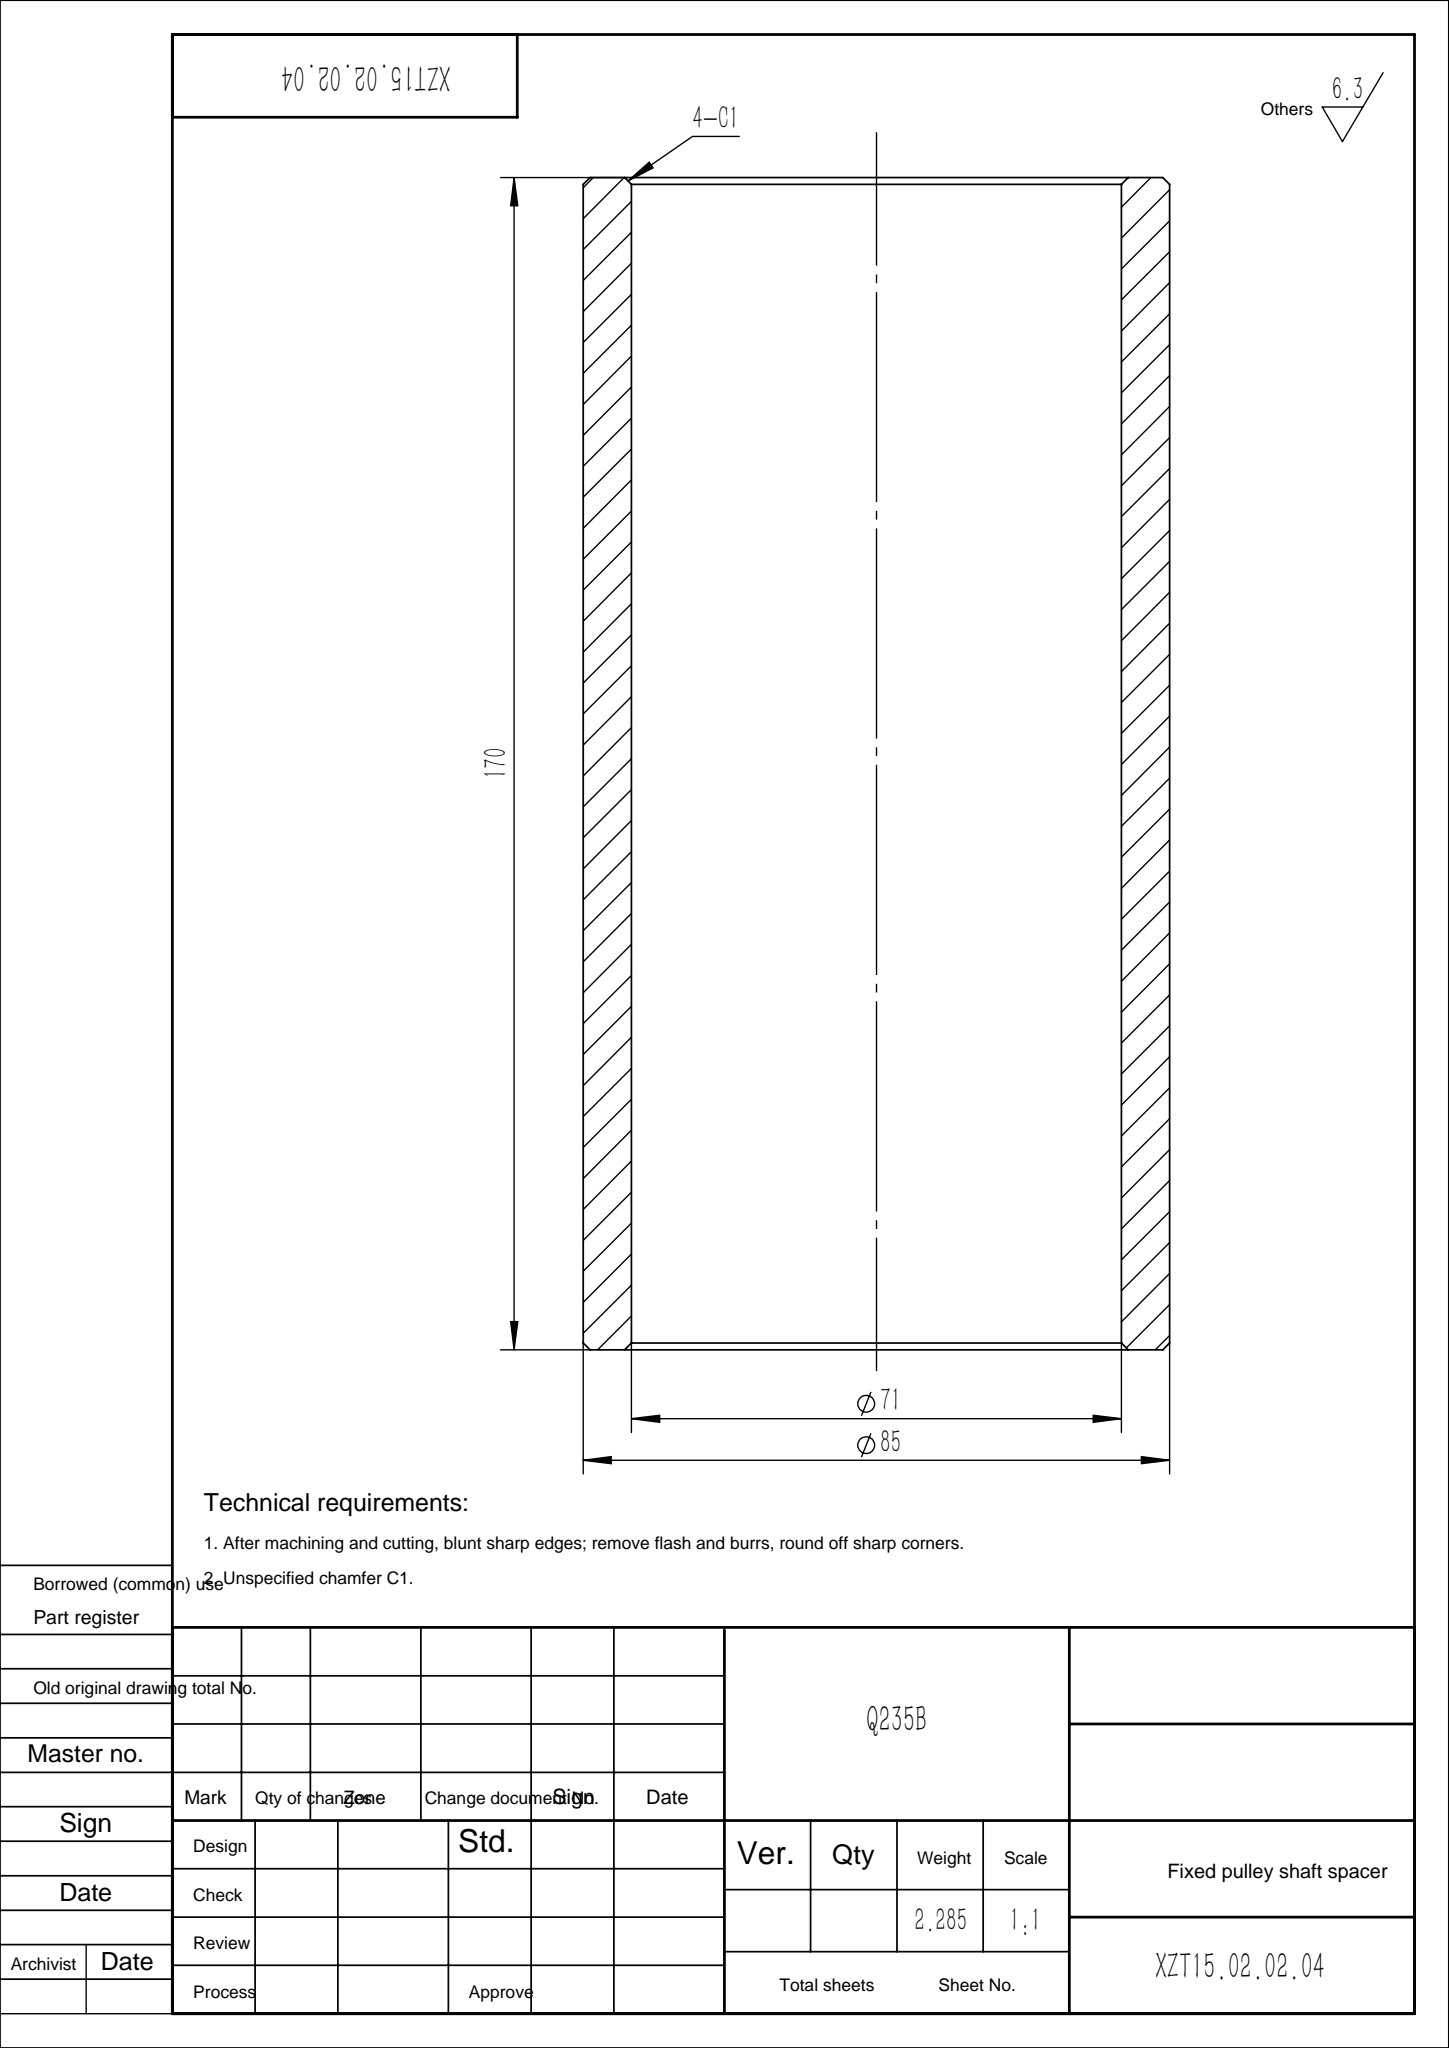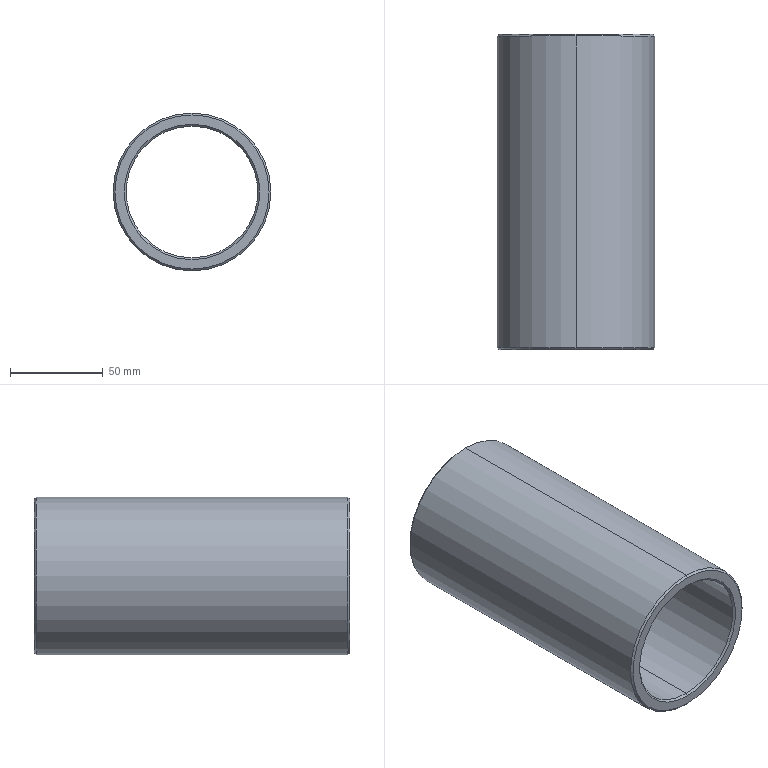Part | SolidWorks | features Chamfer 1, Extrusion 1 | 1 solid | 14 faces | box 85 x 170 x 85 mm | volume 291113 mm3 | cone 8 | cylinder 4 | plane 2 | commonest cylinder face diameters 71 x2 85 x2
STEP:
#1=CARTESIAN_POINT('',(0.,170.,41.5));
#2=VERTEX_POINT('',#1);
#3=CARTESIAN_POINT('',(0.,170.,-41.5));
#4=VERTEX_POINT('',#3);
#5=CARTESIAN_POINT('',(0.,170.,0.));
#6=DIRECTION('',(0.,1.,0.));
#7=DIRECTION('',(0.,0.,1.));
#8=AXIS2_PLACEMENT_3D('',#5,#6,#7);
#9=CIRCLE('',#8,41.5);
#10=EDGE_CURVE('',#2,#4,#9,.T.);
#11=ORIENTED_EDGE('',*,*,#10,.F.);
#12=CARTESIAN_POINT('',(0.,169.,42.5));
#13=VERTEX_POINT('',#12);
#14=CARTESIAN_POINT('',(0.,170.,41.5));
#15=DIRECTION('',(0.,-0.7071,0.7071));
#16=VECTOR('',#15,1000.);
#17=LINE('',#14,#16);
#18=EDGE_CURVE('',#2,#13,#17,.T.);
#19=ORIENTED_EDGE('',*,*,#18,.T.);
#20=CARTESIAN_POINT('',(0.,169.,-42.5));
#21=VERTEX_POINT('',#20);
#22=CARTESIAN_POINT('',(0.,169.,0.));
#23=DIRECTION('',(0.,-1.,0.));
#24=DIRECTION('',(0.,0.,1.));
#25=AXIS2_PLACEMENT_3D('',#22,#23,#24);
#26=CIRCLE('',#25,42.5);
#27=EDGE_CURVE('',#21,#13,#26,.T.);
#28=ORIENTED_EDGE('',*,*,#27,.F.);
#29=CARTESIAN_POINT('',(0.,170.,-41.5));
#30=DIRECTION('',(0.,-0.7071,-0.7071));
#31=VECTOR('',#30,1000.);
#32=LINE('',#29,#31);
#33=EDGE_CURVE('',#4,#21,#32,.T.);
#34=ORIENTED_EDGE('',*,*,#33,.F.);
#35=EDGE_LOOP('',(#11,#19,#28,#34));
#36=FACE_OUTER_BOUND('',#35,.T.);
#37=CARTESIAN_POINT('',(0.,170.,0.));
#38=DIRECTION('',(0.,-1.,0.));
#39=DIRECTION('',(0.,0.,-1.));
#40=AXIS2_PLACEMENT_3D('',#37,#38,#39);
#41=CONICAL_SURFACE('',#40,41.5,0.7854);
#42=ADVANCED_FACE('',(#36),#41,.T.);
#43=CARTESIAN_POINT('',(0.,0.,-41.5));
#44=VERTEX_POINT('',#43);
#45=CARTESIAN_POINT('',(0.,0.,41.5));
#46=VERTEX_POINT('',#45);
#47=CARTESIAN_POINT('',(0.,0.,0.));
#48=DIRECTION('',(0.,-1.,0.));
#49=DIRECTION('',(0.,0.,1.));
#50=AXIS2_PLACEMENT_3D('',#47,#48,#49);
#51=CIRCLE('',#50,41.5);
#52=EDGE_CURVE('',#44,#46,#51,.T.);
#53=ORIENTED_EDGE('',*,*,#52,.F.);
#54=CARTESIAN_POINT('',(0.,1.,-42.5));
#55=VERTEX_POINT('',#54);
#56=CARTESIAN_POINT('',(0.,1.,-42.5));
#57=DIRECTION('',(0.,0.7071,-0.7071));
#58=VECTOR('',#57,1000.);
#59=LINE('',#56,#58);
#60=EDGE_CURVE('',#44,#55,#59,.T.);
#61=ORIENTED_EDGE('',*,*,#60,.T.);
#62=CARTESIAN_POINT('',(0.,1.,42.5));
#63=VERTEX_POINT('',#62);
#64=CARTESIAN_POINT('',(0.,1.,0.));
#65=DIRECTION('',(0.,1.,0.));
#66=DIRECTION('',(0.,0.,1.));
#67=AXIS2_PLACEMENT_3D('',#64,#65,#66);
#68=CIRCLE('',#67,42.5);
#69=EDGE_CURVE('',#63,#55,#68,.T.);
#70=ORIENTED_EDGE('',*,*,#69,.F.);
#71=CARTESIAN_POINT('',(0.,1.,42.5));
#72=DIRECTION('',(0.,0.7071,0.7071));
#73=VECTOR('',#72,1000.);
#74=LINE('',#71,#73);
#75=EDGE_CURVE('',#46,#63,#74,.T.);
#76=ORIENTED_EDGE('',*,*,#75,.F.);
#77=EDGE_LOOP('',(#53,#61,#70,#76));
#78=FACE_OUTER_BOUND('',#77,.T.);
#79=CARTESIAN_POINT('',(0.,1.,0.));
#80=DIRECTION('',(0.,1.,0.));
#81=DIRECTION('',(0.,0.,1.));
#82=AXIS2_PLACEMENT_3D('',#79,#80,#81);
#83=CONICAL_SURFACE('',#82,42.5,0.7854);
#84=ADVANCED_FACE('',(#78),#83,.T.);
#85=CARTESIAN_POINT('',(0.,169.,-35.5));
#86=VERTEX_POINT('',#85);
#87=CARTESIAN_POINT('',(0.,169.,35.5));
#88=VERTEX_POINT('',#87);
#89=CARTESIAN_POINT('',(0.,169.,0.));
#90=DIRECTION('',(0.,1.,0.));
#91=DIRECTION('',(0.,0.,1.));
#92=AXIS2_PLACEMENT_3D('',#89,#90,#91);
#93=CIRCLE('',#92,35.5);
#94=EDGE_CURVE('',#86,#88,#93,.T.);
#95=ORIENTED_EDGE('',*,*,#94,.F.);
#96=CARTESIAN_POINT('',(0.,170.,-36.5));
#97=VERTEX_POINT('',#96);
#98=CARTESIAN_POINT('',(0.,169.,-35.5));
#99=DIRECTION('',(0.,0.7071,-0.7071));
#100=VECTOR('',#99,1000.);
#101=LINE('',#98,#100);
#102=EDGE_CURVE('',#86,#97,#101,.T.);
#103=ORIENTED_EDGE('',*,*,#102,.T.);
#104=CARTESIAN_POINT('',(0.,170.,36.5));
#105=VERTEX_POINT('',#104);
#106=CARTESIAN_POINT('',(0.,170.,0.));
#107=DIRECTION('',(0.,-1.,0.));
#108=DIRECTION('',(0.,0.,1.));
#109=AXIS2_PLACEMENT_3D('',#106,#107,#108);
#110=CIRCLE('',#109,36.5);
#111=EDGE_CURVE('',#105,#97,#110,.T.);
#112=ORIENTED_EDGE('',*,*,#111,.F.);
#113=CARTESIAN_POINT('',(0.,169.,35.5));
#114=DIRECTION('',(0.,0.7071,0.7071));
#115=VECTOR('',#114,1000.);
#116=LINE('',#113,#115);
#117=EDGE_CURVE('',#88,#105,#116,.T.);
#118=ORIENTED_EDGE('',*,*,#117,.F.);
#119=EDGE_LOOP('',(#95,#103,#112,#118));
#120=FACE_OUTER_BOUND('',#119,.T.);
#121=CARTESIAN_POINT('',(0.,169.,0.));
#122=DIRECTION('',(0.,1.,0.));
#123=DIRECTION('',(0.,0.,1.));
#124=AXIS2_PLACEMENT_3D('',#121,#122,#123);
#125=CONICAL_SURFACE('',#124,35.5,0.7854);
#126=ADVANCED_FACE('',(#120),#125,.F.);
#127=CARTESIAN_POINT('',(0.,1.,35.5));
#128=VERTEX_POINT('',#127);
#129=CARTESIAN_POINT('',(0.,1.,-35.5));
#130=VERTEX_POINT('',#129);
#131=CARTESIAN_POINT('',(0.,1.,0.));
#132=DIRECTION('',(0.,-1.,0.));
#133=DIRECTION('',(0.,0.,1.));
#134=AXIS2_PLACEMENT_3D('',#131,#132,#133);
#135=CIRCLE('',#134,35.5);
#136=EDGE_CURVE('',#128,#130,#135,.T.);
#137=ORIENTED_EDGE('',*,*,#136,.F.);
#138=CARTESIAN_POINT('',(0.,0.,36.5));
#139=VERTEX_POINT('',#138);
#140=CARTESIAN_POINT('',(0.,0.,36.5));
#141=DIRECTION('',(0.,-0.7071,0.7071));
#142=VECTOR('',#141,1000.);
#143=LINE('',#140,#142);
#144=EDGE_CURVE('',#128,#139,#143,.T.);
#145=ORIENTED_EDGE('',*,*,#144,.T.);
#146=CARTESIAN_POINT('',(0.,0.,-36.5));
#147=VERTEX_POINT('',#146);
#148=CARTESIAN_POINT('',(0.,0.,0.));
#149=DIRECTION('',(0.,1.,0.));
#150=DIRECTION('',(0.,0.,1.));
#151=AXIS2_PLACEMENT_3D('',#148,#149,#150);
#152=CIRCLE('',#151,36.5);
#153=EDGE_CURVE('',#147,#139,#152,.T.);
#154=ORIENTED_EDGE('',*,*,#153,.F.);
#155=CARTESIAN_POINT('',(0.,0.,-36.5));
#156=DIRECTION('',(0.,-0.7071,-0.7071));
#157=VECTOR('',#156,1000.);
#158=LINE('',#155,#157);
#159=EDGE_CURVE('',#130,#147,#158,.T.);
#160=ORIENTED_EDGE('',*,*,#159,.F.);
#161=EDGE_LOOP('',(#137,#145,#154,#160));
#162=FACE_OUTER_BOUND('',#161,.T.);
#163=CARTESIAN_POINT('',(0.,0.,0.));
#164=DIRECTION('',(0.,-1.,0.));
#165=DIRECTION('',(0.,0.,-1.));
#166=AXIS2_PLACEMENT_3D('',#163,#164,#165);
#167=CONICAL_SURFACE('',#166,36.5,0.7854);
#168=ADVANCED_FACE('',(#162),#167,.F.);
#169=ORIENTED_EDGE('',*,*,#94,.T.);
#170=CARTESIAN_POINT('',(0.,170.,35.5));
#171=DIRECTION('',(0.,-1.,0.));
#172=VECTOR('',#171,1000.);
#173=LINE('',#170,#172);
#174=EDGE_CURVE('',#88,#128,#173,.T.);
#175=ORIENTED_EDGE('',*,*,#174,.T.);
#176=ORIENTED_EDGE('',*,*,#136,.T.);
#177=CARTESIAN_POINT('',(0.,170.,-35.5));
#178=DIRECTION('',(0.,-1.,0.));
#179=VECTOR('',#178,1000.);
#180=LINE('',#177,#179);
#181=EDGE_CURVE('',#86,#130,#180,.T.);
#182=ORIENTED_EDGE('',*,*,#181,.F.);
#183=EDGE_LOOP('',(#169,#175,#176,#182));
#184=FACE_OUTER_BOUND('',#183,.T.);
#185=CARTESIAN_POINT('',(0.,170.,0.));
#186=DIRECTION('',(0.,-1.,0.));
#187=DIRECTION('',(0.,0.,-1.));
#188=AXIS2_PLACEMENT_3D('',#185,#186,#187);
#189=CYLINDRICAL_SURFACE('',#188,35.5);
#190=ADVANCED_FACE('',(#184),#189,.F.);
#191=ORIENTED_EDGE('',*,*,#27,.T.);
#192=CARTESIAN_POINT('',(0.,170.,42.5));
#193=DIRECTION('',(0.,-1.,0.));
#194=VECTOR('',#193,1000.);
#195=LINE('',#192,#194);
#196=EDGE_CURVE('',#13,#63,#195,.T.);
#197=ORIENTED_EDGE('',*,*,#196,.T.);
#198=ORIENTED_EDGE('',*,*,#69,.T.);
#199=CARTESIAN_POINT('',(0.,170.,-42.5));
#200=DIRECTION('',(0.,-1.,0.));
#201=VECTOR('',#200,1000.);
#202=LINE('',#199,#201);
#203=EDGE_CURVE('',#21,#55,#202,.T.);
#204=ORIENTED_EDGE('',*,*,#203,.F.);
#205=EDGE_LOOP('',(#191,#197,#198,#204));
#206=FACE_OUTER_BOUND('',#205,.T.);
#207=CARTESIAN_POINT('',(0.,170.,0.));
#208=DIRECTION('',(0.,-1.,0.));
#209=DIRECTION('',(0.,0.,-1.));
#210=AXIS2_PLACEMENT_3D('',#207,#208,#209);
#211=CYLINDRICAL_SURFACE('',#210,42.5);
#212=ADVANCED_FACE('',(#206),#211,.T.);
#213=ORIENTED_EDGE('',*,*,#111,.T.);
#214=CARTESIAN_POINT('',(0.,170.,0.));
#215=DIRECTION('',(0.,-1.,0.));
#216=DIRECTION('',(0.,0.,1.));
#217=AXIS2_PLACEMENT_3D('',#214,#215,#216);
#218=CIRCLE('',#217,36.5);
#219=EDGE_CURVE('',#97,#105,#218,.T.);
#220=ORIENTED_EDGE('',*,*,#219,.T.);
#221=EDGE_LOOP('',(#213,#220));
#222=FACE_BOUND('',#221,.T.);
#223=CARTESIAN_POINT('',(0.,170.,0.));
#224=DIRECTION('',(0.,1.,0.));
#225=DIRECTION('',(0.,0.,1.));
#226=AXIS2_PLACEMENT_3D('',#223,#224,#225);
#227=CIRCLE('',#226,41.5);
#228=EDGE_CURVE('',#4,#2,#227,.T.);
#229=ORIENTED_EDGE('',*,*,#228,.T.);
#230=ORIENTED_EDGE('',*,*,#10,.T.);
#231=EDGE_LOOP('',(#229,#230));
#232=FACE_OUTER_BOUND('',#231,.T.);
#233=CARTESIAN_POINT('',(0.,170.,0.));
#234=DIRECTION('',(0.,1.,0.));
#235=DIRECTION('',(0.,0.,1.));
#236=AXIS2_PLACEMENT_3D('',#233,#234,#235);
#237=PLANE('',#236);
#238=ADVANCED_FACE('',(#222,#232),#237,.T.);
#239=ORIENTED_EDGE('',*,*,#153,.T.);
#240=CARTESIAN_POINT('',(0.,0.,0.));
#241=DIRECTION('',(0.,1.,0.));
#242=DIRECTION('',(0.,0.,1.));
#243=AXIS2_PLACEMENT_3D('',#240,#241,#242);
#244=CIRCLE('',#243,36.5);
#245=EDGE_CURVE('',#139,#147,#244,.T.);
#246=ORIENTED_EDGE('',*,*,#245,.T.);
#247=EDGE_LOOP('',(#239,#246));
#248=FACE_BOUND('',#247,.T.);
#249=CARTESIAN_POINT('',(0.,0.,0.));
#250=DIRECTION('',(0.,-1.,0.));
#251=DIRECTION('',(0.,0.,1.));
#252=AXIS2_PLACEMENT_3D('',#249,#250,#251);
#253=CIRCLE('',#252,41.5);
#254=EDGE_CURVE('',#46,#44,#253,.T.);
#255=ORIENTED_EDGE('',*,*,#254,.T.);
#256=ORIENTED_EDGE('',*,*,#52,.T.);
#257=EDGE_LOOP('',(#255,#256));
#258=FACE_OUTER_BOUND('',#257,.T.);
#259=CARTESIAN_POINT('',(0.,0.,0.));
#260=DIRECTION('',(0.,1.,0.));
#261=DIRECTION('',(0.,0.,1.));
#262=AXIS2_PLACEMENT_3D('',#259,#260,#261);
#263=PLANE('',#262);
#264=ADVANCED_FACE('',(#248,#258),#263,.F.);
#265=ORIENTED_EDGE('',*,*,#196,.F.);
#266=CARTESIAN_POINT('',(0.,169.,0.));
#267=DIRECTION('',(0.,-1.,0.));
#268=DIRECTION('',(0.,0.,1.));
#269=AXIS2_PLACEMENT_3D('',#266,#267,#268);
#270=CIRCLE('',#269,42.5);
#271=EDGE_CURVE('',#13,#21,#270,.T.);
#272=ORIENTED_EDGE('',*,*,#271,.T.);
#273=ORIENTED_EDGE('',*,*,#203,.T.);
#274=CARTESIAN_POINT('',(0.,1.,0.));
#275=DIRECTION('',(0.,1.,0.));
#276=DIRECTION('',(0.,0.,1.));
#277=AXIS2_PLACEMENT_3D('',#274,#275,#276);
#278=CIRCLE('',#277,42.5);
#279=EDGE_CURVE('',#55,#63,#278,.T.);
#280=ORIENTED_EDGE('',*,*,#279,.T.);
#281=EDGE_LOOP('',(#265,#272,#273,#280));
#282=FACE_OUTER_BOUND('',#281,.T.);
#283=CARTESIAN_POINT('',(0.,170.,0.));
#284=DIRECTION('',(0.,-1.,0.));
#285=DIRECTION('',(0.,0.,-1.));
#286=AXIS2_PLACEMENT_3D('',#283,#284,#285);
#287=CYLINDRICAL_SURFACE('',#286,42.5);
#288=ADVANCED_FACE('',(#282),#287,.T.);
#289=ORIENTED_EDGE('',*,*,#174,.F.);
#290=CARTESIAN_POINT('',(0.,169.,0.));
#291=DIRECTION('',(0.,1.,0.));
#292=DIRECTION('',(0.,0.,1.));
#293=AXIS2_PLACEMENT_3D('',#290,#291,#292);
#294=CIRCLE('',#293,35.5);
#295=EDGE_CURVE('',#88,#86,#294,.T.);
#296=ORIENTED_EDGE('',*,*,#295,.T.);
#297=ORIENTED_EDGE('',*,*,#181,.T.);
#298=CARTESIAN_POINT('',(0.,1.,0.));
#299=DIRECTION('',(0.,-1.,0.));
#300=DIRECTION('',(0.,0.,1.));
#301=AXIS2_PLACEMENT_3D('',#298,#299,#300);
#302=CIRCLE('',#301,35.5);
#303=EDGE_CURVE('',#130,#128,#302,.T.);
#304=ORIENTED_EDGE('',*,*,#303,.T.);
#305=EDGE_LOOP('',(#289,#296,#297,#304));
#306=FACE_OUTER_BOUND('',#305,.T.);
#307=CARTESIAN_POINT('',(0.,170.,0.));
#308=DIRECTION('',(0.,-1.,0.));
#309=DIRECTION('',(0.,0.,-1.));
#310=AXIS2_PLACEMENT_3D('',#307,#308,#309);
#311=CYLINDRICAL_SURFACE('',#310,35.5);
#312=ADVANCED_FACE('',(#306),#311,.F.);
#313=ORIENTED_EDGE('',*,*,#144,.F.);
#314=ORIENTED_EDGE('',*,*,#303,.F.);
#315=ORIENTED_EDGE('',*,*,#159,.T.);
#316=ORIENTED_EDGE('',*,*,#245,.F.);
#317=EDGE_LOOP('',(#313,#314,#315,#316));
#318=FACE_OUTER_BOUND('',#317,.T.);
#319=CARTESIAN_POINT('',(0.,0.,0.));
#320=DIRECTION('',(0.,-1.,0.));
#321=DIRECTION('',(0.,0.,-1.));
#322=AXIS2_PLACEMENT_3D('',#319,#320,#321);
#323=CONICAL_SURFACE('',#322,36.5,0.7854);
#324=ADVANCED_FACE('',(#318),#323,.F.);
#325=ORIENTED_EDGE('',*,*,#102,.F.);
#326=ORIENTED_EDGE('',*,*,#295,.F.);
#327=ORIENTED_EDGE('',*,*,#117,.T.);
#328=ORIENTED_EDGE('',*,*,#219,.F.);
#329=EDGE_LOOP('',(#325,#326,#327,#328));
#330=FACE_OUTER_BOUND('',#329,.T.);
#331=CARTESIAN_POINT('',(0.,169.,0.));
#332=DIRECTION('',(0.,1.,0.));
#333=DIRECTION('',(0.,0.,1.));
#334=AXIS2_PLACEMENT_3D('',#331,#332,#333);
#335=CONICAL_SURFACE('',#334,35.5,0.7854);
#336=ADVANCED_FACE('',(#330),#335,.F.);
#337=ORIENTED_EDGE('',*,*,#60,.F.);
#338=ORIENTED_EDGE('',*,*,#254,.F.);
#339=ORIENTED_EDGE('',*,*,#75,.T.);
#340=ORIENTED_EDGE('',*,*,#279,.F.);
#341=EDGE_LOOP('',(#337,#338,#339,#340));
#342=FACE_OUTER_BOUND('',#341,.T.);
#343=CARTESIAN_POINT('',(0.,1.,0.));
#344=DIRECTION('',(0.,1.,0.));
#345=DIRECTION('',(0.,0.,1.));
#346=AXIS2_PLACEMENT_3D('',#343,#344,#345);
#347=CONICAL_SURFACE('',#346,42.5,0.7854);
#348=ADVANCED_FACE('',(#342),#347,.T.);
#349=ORIENTED_EDGE('',*,*,#18,.F.);
#350=ORIENTED_EDGE('',*,*,#228,.F.);
#351=ORIENTED_EDGE('',*,*,#33,.T.);
#352=ORIENTED_EDGE('',*,*,#271,.F.);
#353=EDGE_LOOP('',(#349,#350,#351,#352));
#354=FACE_OUTER_BOUND('',#353,.T.);
#355=CARTESIAN_POINT('',(0.,170.,0.));
#356=DIRECTION('',(0.,-1.,0.));
#357=DIRECTION('',(0.,0.,-1.));
#358=AXIS2_PLACEMENT_3D('',#355,#356,#357);
#359=CONICAL_SURFACE('',#358,41.5,0.7854);
#360=ADVANCED_FACE('',(#354),#359,.T.);
#361=CLOSED_SHELL('',(#42,#84,#126,#168,#190,#212,#238,#264,#288,#312,#324,#336,#348,#360));
#362=MANIFOLD_SOLID_BREP('',#361);
#363=CARTESIAN_POINT('',(0.,0.,0.));
#364=DIRECTION('',(0.,0.,1.));
#365=DIRECTION('',(1.,0.,0.));
#366=AXIS2_PLACEMENT_3D('',#363,#364,#365);
#367=(LENGTH_UNIT()NAMED_UNIT(*)SI_UNIT(.MILLI.,.METRE.));
#368=UNCERTAINTY_MEASURE_WITH_UNIT(LENGTH_MEASURE(0.00001),#367,'','');
#369=(NAMED_UNIT(*)PLANE_ANGLE_UNIT()SI_UNIT($,.RADIAN.));
#370=(NAMED_UNIT(*)SI_UNIT($,.STERADIAN.)SOLID_ANGLE_UNIT());
#371=(GEOMETRIC_REPRESENTATION_CONTEXT(3)GLOBAL_UNCERTAINTY_ASSIGNED_CONTEXT((#368))GLOBAL_UNIT_ASSIGNED_CONTEXT((#367,#369,#370))REPRESENTATION_CONTEXT('',''));
#372=ADVANCED_BREP_SHAPE_REPRESENTATION('',(#362,#366),#371);